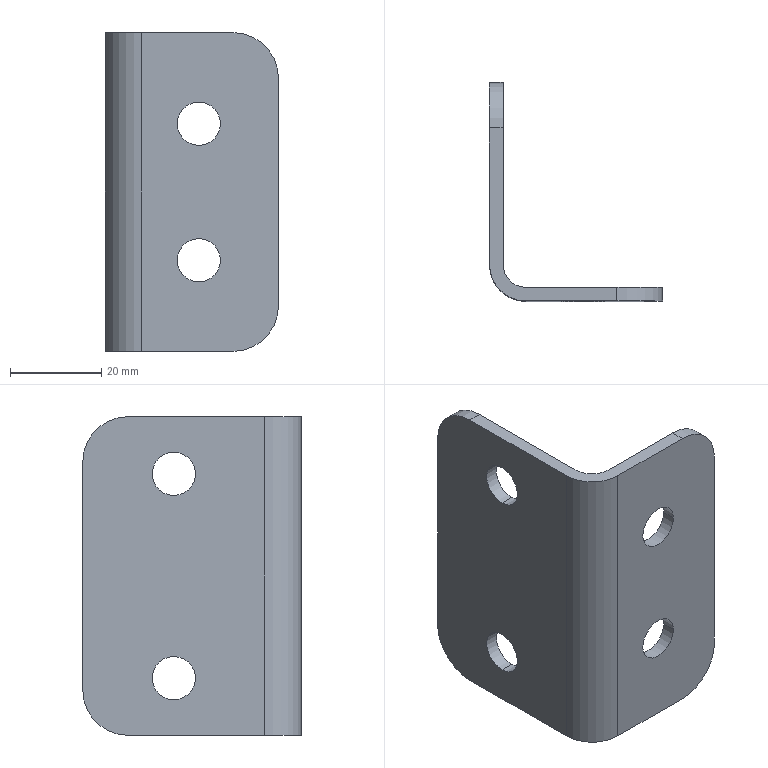Part | STEP file | Part6_5 | 1 solid | 22 faces | box 38 x 48 x 70 mm | volume 15736 mm3 | cylinder 14 | plane 8 | commonest cylinder face diameters 9.5 x4 9.501 x4 20 x4 10 x1 16 x1